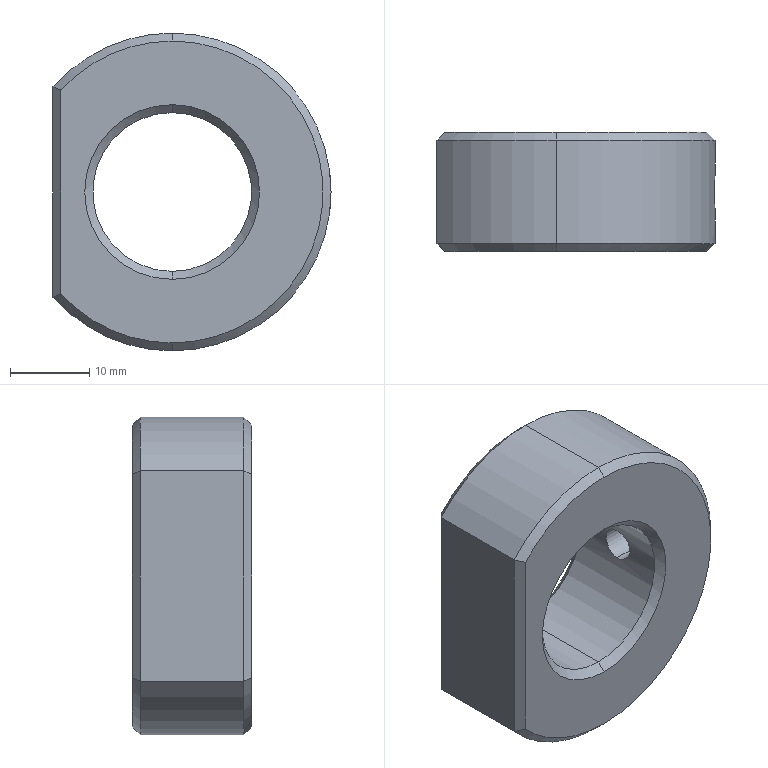Part | SolidWorks | features Chamfer 1, Extrusion 1, HoleWzd 1, ICE 1 | 1 solid | 22 faces | box 35 x 15 x 40 mm | volume 12452 mm3 | cone 10 | cylinder 7 | plane 5 | commonest cylinder face diameters 40 x3 4.2 x2 20 x2
STEP:
#1=CARTESIAN_POINT('',(19.889,7.5,-2.1));
#2=VERTEX_POINT('',#1);
#3=CARTESIAN_POINT('',(19.889,7.5,2.1));
#4=VERTEX_POINT('',#3);
#5=CARTESIAN_POINT('',(19.889,7.5,-2.1));
#6=CARTESIAN_POINT('',(19.889,7.361,-2.1));
#7=CARTESIAN_POINT('',(19.891,7.225,-2.086));
#8=CARTESIAN_POINT('',(19.896,6.956,-2.033));
#9=CARTESIAN_POINT('',(19.901,6.823,-1.993));
#10=CARTESIAN_POINT('',(19.911,6.568,-1.887));
#11=CARTESIAN_POINT('',(19.917,6.448,-1.823));
#12=CARTESIAN_POINT('',(19.93,6.22,-1.67));
#13=CARTESIAN_POINT('',(19.938,6.112,-1.582));
#14=CARTESIAN_POINT('',(19.959,5.821,-1.291));
#15=CARTESIAN_POINT('',(19.974,5.665,-1.057));
#16=CARTESIAN_POINT('',(19.994,5.455,-0.552));
#17=CARTESIAN_POINT('',(20.,5.4,-0.276));
#18=CARTESIAN_POINT('',(20.,5.4,0.1404));
#19=CARTESIAN_POINT('',(19.999,5.414,0.2768));
#20=CARTESIAN_POINT('',(19.993,5.467,0.5453));
#21=CARTESIAN_POINT('',(19.989,5.508,0.6787));
#22=CARTESIAN_POINT('',(19.979,5.614,0.9328));
#23=CARTESIAN_POINT('',(19.973,5.678,1.053));
#24=CARTESIAN_POINT('',(19.959,5.831,1.281));
#25=CARTESIAN_POINT('',(19.952,5.919,1.389));
#26=CARTESIAN_POINT('',(19.93,6.21,1.679));
#27=CARTESIAN_POINT('',(19.916,6.444,1.836));
#28=CARTESIAN_POINT('',(19.895,6.949,2.045));
#29=CARTESIAN_POINT('',(19.889,7.226,2.1));
#30=CARTESIAN_POINT('',(19.889,7.5,2.1));
#31=B_SPLINE_CURVE_WITH_KNOTS('',3,(#5,#6,#7,#8,#9,#10,#11,#12,#13,#14,#15,#16,#17,#18,#19,#20,#21,#22,#23,#24,#25,#26,#27,#28,#29,#30),.UNSPECIFIED.,.F.,.F.,(4,2,2,2,2,2,2,2,2,2,2,2,4),(0.009856,0.01027,0.01068,0.01109,0.0115,0.01232,0.01314,0.01355,0.01396,0.01437,0.01478,0.0156,0.01642),.UNSPECIFIED.);
#32=EDGE_CURVE('',#2,#4,#31,.T.);
#33=ORIENTED_EDGE('',*,*,#32,.F.);
#34=CARTESIAN_POINT('',(9.777,7.5,-2.1));
#35=VERTEX_POINT('',#34);
#36=CARTESIAN_POINT('',(0.,7.5,-2.1));
#37=DIRECTION('',(-1.,0.,0.));
#38=VECTOR('',#37,1000.);
#39=LINE('',#36,#38);
#40=EDGE_CURVE('',#2,#35,#39,.T.);
#41=ORIENTED_EDGE('',*,*,#40,.T.);
#42=CARTESIAN_POINT('',(9.777,7.5,2.1));
#43=VERTEX_POINT('',#42);
#44=CARTESIAN_POINT('',(9.777,7.5,-2.1));
#45=CARTESIAN_POINT('',(9.777,7.226,-2.1));
#46=CARTESIAN_POINT('',(9.789,6.949,-2.045));
#47=CARTESIAN_POINT('',(9.82,6.569,-1.887));
#48=CARTESIAN_POINT('',(9.833,6.447,-1.822));
#49=CARTESIAN_POINT('',(9.86,6.218,-1.669));
#50=CARTESIAN_POINT('',(9.874,6.113,-1.583));
#51=CARTESIAN_POINT('',(9.904,5.919,-1.389));
#52=CARTESIAN_POINT('',(9.918,5.831,-1.281));
#53=CARTESIAN_POINT('',(9.945,5.679,-1.054));
#54=CARTESIAN_POINT('',(9.957,5.614,-0.9337));
#55=CARTESIAN_POINT('',(9.988,5.455,-0.5514));
#56=CARTESIAN_POINT('',(10.,5.4,-0.2782));
#57=CARTESIAN_POINT('',(10.,5.4,0.1376));
#58=CARTESIAN_POINT('',(9.997,5.413,0.2742));
#59=CARTESIAN_POINT('',(9.986,5.467,0.5435));
#60=CARTESIAN_POINT('',(9.978,5.508,0.6774));
#61=CARTESIAN_POINT('',(9.957,5.613,0.931));
#62=CARTESIAN_POINT('',(9.945,5.677,1.052));
#63=CARTESIAN_POINT('',(9.918,5.83,1.28));
#64=CARTESIAN_POINT('',(9.904,5.918,1.388));
#65=CARTESIAN_POINT('',(9.86,6.207,1.677));
#66=CARTESIAN_POINT('',(9.831,6.441,1.834));
#67=CARTESIAN_POINT('',(9.8,6.819,1.991));
#68=CARTESIAN_POINT('',(9.791,6.953,2.032));
#69=CARTESIAN_POINT('',(9.78,7.224,2.086));
#70=CARTESIAN_POINT('',(9.777,7.361,2.1));
#71=CARTESIAN_POINT('',(9.777,7.5,2.1));
#72=B_SPLINE_CURVE_WITH_KNOTS('',3,(#44,#45,#46,#47,#48,#49,#50,#51,#52,#53,#54,#55,#56,#57,#58,#59,#60,#61,#62,#63,#64,#65,#66,#67,#68,#69,#70,#71),.UNSPECIFIED.,.F.,.F.,(4,2,2,2,2,2,2,2,2,2,2,2,2,4),(0.006584,0.007407,0.007818,0.008229,0.008641,0.009052,0.009875,0.01029,0.0107,0.01111,0.01152,0.01234,0.01275,0.01317),.UNSPECIFIED.);
#73=EDGE_CURVE('',#35,#43,#72,.T.);
#74=ORIENTED_EDGE('',*,*,#73,.T.);
#75=CARTESIAN_POINT('',(0.,7.5,2.1));
#76=DIRECTION('',(-1.,0.,0.));
#77=VECTOR('',#76,1000.);
#78=LINE('',#75,#77);
#79=EDGE_CURVE('',#4,#43,#78,.T.);
#80=ORIENTED_EDGE('',*,*,#79,.F.);
#81=EDGE_LOOP('',(#33,#41,#74,#80));
#82=FACE_OUTER_BOUND('',#81,.T.);
#83=CARTESIAN_POINT('',(0.,7.5,0.));
#84=DIRECTION('',(-1.,0.,0.));
#85=DIRECTION('',(0.,0.,1.));
#86=AXIS2_PLACEMENT_3D('',#83,#84,#85);
#87=CYLINDRICAL_SURFACE('',#86,2.1);
#88=ADVANCED_FACE('',(#82),#87,.F.);
#89=CARTESIAN_POINT('',(0.,15.,19.));
#90=VERTEX_POINT('',#89);
#91=CARTESIAN_POINT('',(0.,15.,-19.));
#92=VERTEX_POINT('',#91);
#93=CARTESIAN_POINT('',(0.,15.,0.));
#94=DIRECTION('',(0.,1.,0.));
#95=DIRECTION('',(0.,0.,1.));
#96=AXIS2_PLACEMENT_3D('',#93,#94,#95);
#97=CIRCLE('',#96,19.);
#98=EDGE_CURVE('',#90,#92,#97,.T.);
#99=ORIENTED_EDGE('',*,*,#98,.F.);
#100=CARTESIAN_POINT('',(0.,14.,20.));
#101=VERTEX_POINT('',#100);
#102=CARTESIAN_POINT('',(0.,15.,19.));
#103=DIRECTION('',(0.,-0.7071,0.7071));
#104=VECTOR('',#103,1000.);
#105=LINE('',#102,#104);
#106=EDGE_CURVE('',#90,#101,#105,.T.);
#107=ORIENTED_EDGE('',*,*,#106,.T.);
#108=CARTESIAN_POINT('',(0.,14.,-20.));
#109=VERTEX_POINT('',#108);
#110=CARTESIAN_POINT('',(0.,14.,0.));
#111=DIRECTION('',(0.,-1.,0.));
#112=DIRECTION('',(0.,0.,1.));
#113=AXIS2_PLACEMENT_3D('',#110,#111,#112);
#114=CIRCLE('',#113,20.);
#115=EDGE_CURVE('',#109,#101,#114,.T.);
#116=ORIENTED_EDGE('',*,*,#115,.F.);
#117=CARTESIAN_POINT('',(0.,15.,-19.));
#118=DIRECTION('',(0.,-0.7071,-0.7071));
#119=VECTOR('',#118,1000.);
#120=LINE('',#117,#119);
#121=EDGE_CURVE('',#92,#109,#120,.T.);
#122=ORIENTED_EDGE('',*,*,#121,.F.);
#123=EDGE_LOOP('',(#99,#107,#116,#122));
#124=FACE_OUTER_BOUND('',#123,.T.);
#125=CARTESIAN_POINT('',(0.,15.,0.));
#126=DIRECTION('',(0.,-1.,0.));
#127=DIRECTION('',(0.,0.,-1.));
#128=AXIS2_PLACEMENT_3D('',#125,#126,#127);
#129=CONICAL_SURFACE('',#128,19.,0.7854);
#130=ADVANCED_FACE('',(#124),#129,.T.);
#131=CARTESIAN_POINT('',(-14.,15.,-12.845));
#132=VERTEX_POINT('',#131);
#133=CARTESIAN_POINT('',(0.,15.,0.));
#134=DIRECTION('',(0.,1.,0.));
#135=DIRECTION('',(0.,0.,1.));
#136=AXIS2_PLACEMENT_3D('',#133,#134,#135);
#137=CIRCLE('',#136,19.);
#138=EDGE_CURVE('',#92,#132,#137,.T.);
#139=ORIENTED_EDGE('',*,*,#138,.F.);
#140=ORIENTED_EDGE('',*,*,#121,.T.);
#141=CARTESIAN_POINT('',(-15.,14.,-13.229));
#142=VERTEX_POINT('',#141);
#143=CARTESIAN_POINT('',(0.,14.,0.));
#144=DIRECTION('',(0.,-1.,0.));
#145=DIRECTION('',(0.,0.,1.));
#146=AXIS2_PLACEMENT_3D('',#143,#144,#145);
#147=CIRCLE('',#146,20.);
#148=EDGE_CURVE('',#142,#109,#147,.T.);
#149=ORIENTED_EDGE('',*,*,#148,.F.);
#150=CARTESIAN_POINT('',(-14.,15.,-12.845));
#151=CARTESIAN_POINT('',(-14.333,14.667,-12.975));
#152=CARTESIAN_POINT('',(-14.666,14.334,-13.103));
#153=CARTESIAN_POINT('',(-15.,14.,-13.229));
#154=B_SPLINE_CURVE_WITH_KNOTS('',3,(#150,#151,#152,#153),.UNSPECIFIED.,.F.,.F.,(4,4),(0.,0.001465),.UNSPECIFIED.);
#155=EDGE_CURVE('',#132,#142,#154,.T.);
#156=ORIENTED_EDGE('',*,*,#155,.F.);
#157=EDGE_LOOP('',(#139,#140,#149,#156));
#158=FACE_OUTER_BOUND('',#157,.T.);
#159=CARTESIAN_POINT('',(0.,15.,0.));
#160=DIRECTION('',(0.,-1.,0.));
#161=DIRECTION('',(0.,0.,-1.));
#162=AXIS2_PLACEMENT_3D('',#159,#160,#161);
#163=CONICAL_SURFACE('',#162,19.,0.7854);
#164=ADVANCED_FACE('',(#158),#163,.T.);
#165=CARTESIAN_POINT('',(0.,0.,-19.));
#166=VERTEX_POINT('',#165);
#167=CARTESIAN_POINT('',(0.,0.,19.));
#168=VERTEX_POINT('',#167);
#169=CARTESIAN_POINT('',(0.,0.,0.));
#170=DIRECTION('',(0.,-1.,0.));
#171=DIRECTION('',(0.,0.,1.));
#172=AXIS2_PLACEMENT_3D('',#169,#170,#171);
#173=CIRCLE('',#172,19.);
#174=EDGE_CURVE('',#166,#168,#173,.T.);
#175=ORIENTED_EDGE('',*,*,#174,.F.);
#176=CARTESIAN_POINT('',(0.,1.,-20.));
#177=VERTEX_POINT('',#176);
#178=CARTESIAN_POINT('',(0.,1.,-20.));
#179=DIRECTION('',(0.,0.7071,-0.7071));
#180=VECTOR('',#179,1000.);
#181=LINE('',#178,#180);
#182=EDGE_CURVE('',#166,#177,#181,.T.);
#183=ORIENTED_EDGE('',*,*,#182,.T.);
#184=CARTESIAN_POINT('',(0.,1.,20.));
#185=VERTEX_POINT('',#184);
#186=CARTESIAN_POINT('',(0.,1.,0.));
#187=DIRECTION('',(0.,1.,0.));
#188=DIRECTION('',(0.,0.,1.));
#189=AXIS2_PLACEMENT_3D('',#186,#187,#188);
#190=CIRCLE('',#189,20.);
#191=EDGE_CURVE('',#185,#177,#190,.T.);
#192=ORIENTED_EDGE('',*,*,#191,.F.);
#193=CARTESIAN_POINT('',(0.,1.,20.));
#194=DIRECTION('',(0.,0.7071,0.7071));
#195=VECTOR('',#194,1000.);
#196=LINE('',#193,#195);
#197=EDGE_CURVE('',#168,#185,#196,.T.);
#198=ORIENTED_EDGE('',*,*,#197,.F.);
#199=EDGE_LOOP('',(#175,#183,#192,#198));
#200=FACE_OUTER_BOUND('',#199,.T.);
#201=CARTESIAN_POINT('',(0.,1.,0.));
#202=DIRECTION('',(0.,1.,0.));
#203=DIRECTION('',(0.,0.,1.));
#204=AXIS2_PLACEMENT_3D('',#201,#202,#203);
#205=CONICAL_SURFACE('',#204,20.,0.7854);
#206=ADVANCED_FACE('',(#200),#205,.T.);
#207=CARTESIAN_POINT('',(-14.,0.,12.845));
#208=VERTEX_POINT('',#207);
#209=CARTESIAN_POINT('',(0.,0.,0.));
#210=DIRECTION('',(0.,-1.,0.));
#211=DIRECTION('',(0.,0.,1.));
#212=AXIS2_PLACEMENT_3D('',#209,#210,#211);
#213=CIRCLE('',#212,19.);
#214=EDGE_CURVE('',#168,#208,#213,.T.);
#215=ORIENTED_EDGE('',*,*,#214,.F.);
#216=ORIENTED_EDGE('',*,*,#197,.T.);
#217=CARTESIAN_POINT('',(-15.,1.,13.229));
#218=VERTEX_POINT('',#217);
#219=CARTESIAN_POINT('',(0.,1.,0.));
#220=DIRECTION('',(0.,1.,0.));
#221=DIRECTION('',(0.,0.,1.));
#222=AXIS2_PLACEMENT_3D('',#219,#220,#221);
#223=CIRCLE('',#222,20.);
#224=EDGE_CURVE('',#218,#185,#223,.T.);
#225=ORIENTED_EDGE('',*,*,#224,.F.);
#226=CARTESIAN_POINT('',(-14.,0.,12.845));
#227=CARTESIAN_POINT('',(-14.333,0.333,12.975));
#228=CARTESIAN_POINT('',(-14.666,0.6663,13.103));
#229=CARTESIAN_POINT('',(-15.,1.,13.229));
#230=B_SPLINE_CURVE_WITH_KNOTS('',3,(#226,#227,#228,#229),.UNSPECIFIED.,.F.,.F.,(4,4),(0.,0.001465),.UNSPECIFIED.);
#231=EDGE_CURVE('',#208,#218,#230,.T.);
#232=ORIENTED_EDGE('',*,*,#231,.F.);
#233=EDGE_LOOP('',(#215,#216,#225,#232));
#234=FACE_OUTER_BOUND('',#233,.T.);
#235=CARTESIAN_POINT('',(0.,1.,0.));
#236=DIRECTION('',(0.,1.,0.));
#237=DIRECTION('',(0.,0.,1.));
#238=AXIS2_PLACEMENT_3D('',#235,#236,#237);
#239=CONICAL_SURFACE('',#238,20.,0.7854);
#240=ADVANCED_FACE('',(#234),#239,.T.);
#241=CARTESIAN_POINT('',(0.,14.,-10.));
#242=VERTEX_POINT('',#241);
#243=CARTESIAN_POINT('',(0.,14.,10.));
#244=VERTEX_POINT('',#243);
#245=CARTESIAN_POINT('',(0.,14.,0.));
#246=DIRECTION('',(0.,1.,0.));
#247=DIRECTION('',(0.,0.,1.));
#248=AXIS2_PLACEMENT_3D('',#245,#246,#247);
#249=CIRCLE('',#248,10.);
#250=EDGE_CURVE('',#242,#244,#249,.T.);
#251=ORIENTED_EDGE('',*,*,#250,.F.);
#252=CARTESIAN_POINT('',(0.,15.,-11.));
#253=VERTEX_POINT('',#252);
#254=CARTESIAN_POINT('',(0.,14.,-10.));
#255=DIRECTION('',(0.,0.7071,-0.7071));
#256=VECTOR('',#255,1000.);
#257=LINE('',#254,#256);
#258=EDGE_CURVE('',#242,#253,#257,.T.);
#259=ORIENTED_EDGE('',*,*,#258,.T.);
#260=CARTESIAN_POINT('',(0.,15.,11.));
#261=VERTEX_POINT('',#260);
#262=CARTESIAN_POINT('',(0.,15.,0.));
#263=DIRECTION('',(0.,-1.,0.));
#264=DIRECTION('',(0.,0.,1.));
#265=AXIS2_PLACEMENT_3D('',#262,#263,#264);
#266=CIRCLE('',#265,11.);
#267=EDGE_CURVE('',#261,#253,#266,.T.);
#268=ORIENTED_EDGE('',*,*,#267,.F.);
#269=CARTESIAN_POINT('',(0.,14.,10.));
#270=DIRECTION('',(0.,0.7071,0.7071));
#271=VECTOR('',#270,1000.);
#272=LINE('',#269,#271);
#273=EDGE_CURVE('',#244,#261,#272,.T.);
#274=ORIENTED_EDGE('',*,*,#273,.F.);
#275=EDGE_LOOP('',(#251,#259,#268,#274));
#276=FACE_OUTER_BOUND('',#275,.T.);
#277=CARTESIAN_POINT('',(0.,14.,0.));
#278=DIRECTION('',(0.,1.,0.));
#279=DIRECTION('',(0.,0.,1.));
#280=AXIS2_PLACEMENT_3D('',#277,#278,#279);
#281=CONICAL_SURFACE('',#280,10.,0.7854);
#282=ADVANCED_FACE('',(#276),#281,.F.);
#283=CARTESIAN_POINT('',(0.,1.,10.));
#284=VERTEX_POINT('',#283);
#285=CARTESIAN_POINT('',(0.,1.,-10.));
#286=VERTEX_POINT('',#285);
#287=CARTESIAN_POINT('',(0.,1.,0.));
#288=DIRECTION('',(0.,-1.,0.));
#289=DIRECTION('',(0.,0.,1.));
#290=AXIS2_PLACEMENT_3D('',#287,#288,#289);
#291=CIRCLE('',#290,10.);
#292=EDGE_CURVE('',#284,#286,#291,.T.);
#293=ORIENTED_EDGE('',*,*,#292,.F.);
#294=CARTESIAN_POINT('',(0.,0.,11.));
#295=VERTEX_POINT('',#294);
#296=CARTESIAN_POINT('',(0.,0.,11.));
#297=DIRECTION('',(0.,-0.7071,0.7071));
#298=VECTOR('',#297,1000.);
#299=LINE('',#296,#298);
#300=EDGE_CURVE('',#284,#295,#299,.T.);
#301=ORIENTED_EDGE('',*,*,#300,.T.);
#302=CARTESIAN_POINT('',(0.,0.,-11.));
#303=VERTEX_POINT('',#302);
#304=CARTESIAN_POINT('',(0.,0.,0.));
#305=DIRECTION('',(0.,1.,0.));
#306=DIRECTION('',(0.,0.,1.));
#307=AXIS2_PLACEMENT_3D('',#304,#305,#306);
#308=CIRCLE('',#307,11.);
#309=EDGE_CURVE('',#303,#295,#308,.T.);
#310=ORIENTED_EDGE('',*,*,#309,.F.);
#311=CARTESIAN_POINT('',(0.,0.,-11.));
#312=DIRECTION('',(0.,-0.7071,-0.7071));
#313=VECTOR('',#312,1000.);
#314=LINE('',#311,#313);
#315=EDGE_CURVE('',#286,#303,#314,.T.);
#316=ORIENTED_EDGE('',*,*,#315,.F.);
#317=EDGE_LOOP('',(#293,#301,#310,#316));
#318=FACE_OUTER_BOUND('',#317,.T.);
#319=CARTESIAN_POINT('',(0.,0.,0.));
#320=DIRECTION('',(0.,-1.,0.));
#321=DIRECTION('',(0.,0.,-1.));
#322=AXIS2_PLACEMENT_3D('',#319,#320,#321);
#323=CONICAL_SURFACE('',#322,11.,0.7854);
#324=ADVANCED_FACE('',(#318),#323,.F.);
#325=ORIENTED_EDGE('',*,*,#250,.T.);
#326=CARTESIAN_POINT('',(0.,15.,10.));
#327=DIRECTION('',(0.,-1.,0.));
#328=VECTOR('',#327,1000.);
#329=LINE('',#326,#328);
#330=EDGE_CURVE('',#244,#284,#329,.T.);
#331=ORIENTED_EDGE('',*,*,#330,.T.);
#332=ORIENTED_EDGE('',*,*,#292,.T.);
#333=CARTESIAN_POINT('',(0.,15.,-10.));
#334=DIRECTION('',(0.,-1.,0.));
#335=VECTOR('',#334,1000.);
#336=LINE('',#333,#335);
#337=EDGE_CURVE('',#242,#286,#336,.T.);
#338=ORIENTED_EDGE('',*,*,#337,.F.);
#339=EDGE_LOOP('',(#325,#331,#332,#338));
#340=FACE_OUTER_BOUND('',#339,.T.);
#341=CARTESIAN_POINT('',(0.,15.,0.));
#342=DIRECTION('',(0.,-1.,0.));
#343=DIRECTION('',(0.,0.,-1.));
#344=AXIS2_PLACEMENT_3D('',#341,#342,#343);
#345=CYLINDRICAL_SURFACE('',#344,10.);
#346=ADVANCED_FACE('',(#340),#345,.F.);
#347=CARTESIAN_POINT('',(19.889,7.5,2.1));
#348=CARTESIAN_POINT('',(19.889,7.637,2.1));
#349=CARTESIAN_POINT('',(19.891,7.776,2.086));
#350=CARTESIAN_POINT('',(19.896,8.046,2.033));
#351=CARTESIAN_POINT('',(19.901,8.177,1.993));
#352=CARTESIAN_POINT('',(19.911,8.431,1.887));
#353=CARTESIAN_POINT('',(19.917,8.554,1.822));
#354=CARTESIAN_POINT('',(19.93,8.781,1.669));
#355=CARTESIAN_POINT('',(19.938,8.887,1.583));
#356=CARTESIAN_POINT('',(19.952,9.083,1.387));
#357=CARTESIAN_POINT('',(19.959,9.17,1.281));
#358=CARTESIAN_POINT('',(19.973,9.322,1.053));
#359=CARTESIAN_POINT('',(19.979,9.388,0.9302));
#360=CARTESIAN_POINT('',(19.989,9.493,0.6759));
#361=CARTESIAN_POINT('',(19.993,9.533,0.5449));
#362=CARTESIAN_POINT('',(19.999,9.586,0.2756));
#363=CARTESIAN_POINT('',(20.,9.6,0.1363));
#364=CARTESIAN_POINT('',(20.,9.6,-0.275));
#365=CARTESIAN_POINT('',(19.994,9.545,-0.5515));
#366=CARTESIAN_POINT('',(19.974,9.335,-1.057));
#367=CARTESIAN_POINT('',(19.959,9.179,-1.291));
#368=CARTESIAN_POINT('',(19.938,8.888,-1.582));
#369=CARTESIAN_POINT('',(19.93,8.78,-1.67));
#370=CARTESIAN_POINT('',(19.917,8.552,-1.823));
#371=CARTESIAN_POINT('',(19.911,8.432,-1.887));
#372=CARTESIAN_POINT('',(19.901,8.177,-1.993));
#373=CARTESIAN_POINT('',(19.896,8.044,-2.033));
#374=CARTESIAN_POINT('',(19.891,7.775,-2.086));
#375=CARTESIAN_POINT('',(19.889,7.639,-2.1));
#376=CARTESIAN_POINT('',(19.889,7.5,-2.1));
#377=B_SPLINE_CURVE_WITH_KNOTS('',3,(#347,#348,#349,#350,#351,#352,#353,#354,#355,#356,#357,#358,#359,#360,#361,#362,#363,#364,#365,#366,#367,#368,#369,#370,#371,#372,#373,#374,#375,#376),.UNSPECIFIED.,.F.,.F.,(4,2,2,2,2,2,2,2,2,2,2,2,2,2,4),(0.003286,0.003696,0.004107,0.004518,0.004928,0.005339,0.00575,0.00616,0.006571,0.007392,0.008213,0.008624,0.009035,0.009445,0.009856),.UNSPECIFIED.);
#378=EDGE_CURVE('',#4,#2,#377,.T.);
#379=ORIENTED_EDGE('',*,*,#378,.T.);
#380=ORIENTED_EDGE('',*,*,#32,.T.);
#381=EDGE_LOOP('',(#379,#380));
#382=FACE_BOUND('',#381,.T.);
#383=ORIENTED_EDGE('',*,*,#115,.T.);
#384=CARTESIAN_POINT('',(0.,15.,20.));
#385=DIRECTION('',(0.,-1.,0.));
#386=VECTOR('',#385,1000.);
#387=LINE('',#384,#386);
#388=EDGE_CURVE('',#101,#185,#387,.T.);
#389=ORIENTED_EDGE('',*,*,#388,.T.);
#390=ORIENTED_EDGE('',*,*,#191,.T.);
#391=CARTESIAN_POINT('',(0.,15.,-20.));
#392=DIRECTION('',(0.,-1.,0.));
#393=VECTOR('',#392,1000.);
#394=LINE('',#391,#393);
#395=EDGE_CURVE('',#109,#177,#394,.T.);
#396=ORIENTED_EDGE('',*,*,#395,.F.);
#397=EDGE_LOOP('',(#383,#389,#390,#396));
#398=FACE_OUTER_BOUND('',#397,.T.);
#399=CARTESIAN_POINT('',(0.,15.,0.));
#400=DIRECTION('',(0.,-1.,0.));
#401=DIRECTION('',(0.,0.,-1.));
#402=AXIS2_PLACEMENT_3D('',#399,#400,#401);
#403=CYLINDRICAL_SURFACE('',#402,20.);
#404=ADVANCED_FACE('',(#382,#398),#403,.T.);
#405=ORIENTED_EDGE('',*,*,#148,.T.);
#406=ORIENTED_EDGE('',*,*,#395,.T.);
#407=CARTESIAN_POINT('',(-15.,1.,-13.229));
#408=VERTEX_POINT('',#407);
#409=CARTESIAN_POINT('',(0.,1.,0.));
#410=DIRECTION('',(0.,1.,0.));
#411=DIRECTION('',(0.,0.,1.));
#412=AXIS2_PLACEMENT_3D('',#409,#410,#411);
#413=CIRCLE('',#412,20.);
#414=EDGE_CURVE('',#177,#408,#413,.T.);
#415=ORIENTED_EDGE('',*,*,#414,.T.);
#416=CARTESIAN_POINT('',(-15.,15.,-13.229));
#417=DIRECTION('',(0.,1.,0.));
#418=VECTOR('',#417,1000.);
#419=LINE('',#416,#418);
#420=EDGE_CURVE('',#408,#142,#419,.T.);
#421=ORIENTED_EDGE('',*,*,#420,.T.);
#422=EDGE_LOOP('',(#405,#406,#415,#421));
#423=FACE_OUTER_BOUND('',#422,.T.);
#424=CARTESIAN_POINT('',(0.,15.,0.));
#425=DIRECTION('',(0.,-1.,0.));
#426=DIRECTION('',(0.,0.,-1.));
#427=AXIS2_PLACEMENT_3D('',#424,#425,#426);
#428=CYLINDRICAL_SURFACE('',#427,20.);
#429=ADVANCED_FACE('',(#423),#428,.T.);
#430=ORIENTED_EDGE('',*,*,#267,.T.);
#431=CARTESIAN_POINT('',(0.,15.,0.));
#432=DIRECTION('',(0.,-1.,0.));
#433=DIRECTION('',(0.,0.,1.));
#434=AXIS2_PLACEMENT_3D('',#431,#432,#433);
#435=CIRCLE('',#434,11.);
#436=EDGE_CURVE('',#253,#261,#435,.T.);
#437=ORIENTED_EDGE('',*,*,#436,.T.);
#438=EDGE_LOOP('',(#430,#437));
#439=FACE_BOUND('',#438,.T.);
#440=CARTESIAN_POINT('',(-14.,15.,12.845));
#441=VERTEX_POINT('',#440);
#442=CARTESIAN_POINT('',(0.,15.,0.));
#443=DIRECTION('',(0.,1.,0.));
#444=DIRECTION('',(0.,0.,1.));
#445=AXIS2_PLACEMENT_3D('',#442,#443,#444);
#446=CIRCLE('',#445,19.);
#447=EDGE_CURVE('',#441,#90,#446,.T.);
#448=ORIENTED_EDGE('',*,*,#447,.T.);
#449=ORIENTED_EDGE('',*,*,#98,.T.);
#450=ORIENTED_EDGE('',*,*,#138,.T.);
#451=CARTESIAN_POINT('',(-14.,15.,13.229));
#452=DIRECTION('',(0.,0.,1.));
#453=VECTOR('',#452,1000.);
#454=LINE('',#451,#453);
#455=EDGE_CURVE('',#132,#441,#454,.T.);
#456=ORIENTED_EDGE('',*,*,#455,.T.);
#457=EDGE_LOOP('',(#448,#449,#450,#456));
#458=FACE_OUTER_BOUND('',#457,.T.);
#459=CARTESIAN_POINT('',(0.,15.,0.));
#460=DIRECTION('',(0.,1.,0.));
#461=DIRECTION('',(0.,0.,1.));
#462=AXIS2_PLACEMENT_3D('',#459,#460,#461);
#463=PLANE('',#462);
#464=ADVANCED_FACE('',(#439,#458),#463,.T.);
#465=ORIENTED_EDGE('',*,*,#309,.T.);
#466=CARTESIAN_POINT('',(0.,0.,0.));
#467=DIRECTION('',(0.,1.,0.));
#468=DIRECTION('',(0.,0.,1.));
#469=AXIS2_PLACEMENT_3D('',#466,#467,#468);
#470=CIRCLE('',#469,11.);
#471=EDGE_CURVE('',#295,#303,#470,.T.);
#472=ORIENTED_EDGE('',*,*,#471,.T.);
#473=EDGE_LOOP('',(#465,#472));
#474=FACE_BOUND('',#473,.T.);
#475=CARTESIAN_POINT('',(-14.,0.,-12.845));
#476=VERTEX_POINT('',#475);
#477=CARTESIAN_POINT('',(0.,0.,0.));
#478=DIRECTION('',(0.,-1.,0.));
#479=DIRECTION('',(0.,0.,1.));
#480=AXIS2_PLACEMENT_3D('',#477,#478,#479);
#481=CIRCLE('',#480,19.);
#482=EDGE_CURVE('',#476,#166,#481,.T.);
#483=ORIENTED_EDGE('',*,*,#482,.T.);
#484=ORIENTED_EDGE('',*,*,#174,.T.);
#485=ORIENTED_EDGE('',*,*,#214,.T.);
#486=CARTESIAN_POINT('',(-14.,0.,0.));
#487=DIRECTION('',(0.,0.,-1.));
#488=VECTOR('',#487,1000.);
#489=LINE('',#486,#488);
#490=EDGE_CURVE('',#208,#476,#489,.T.);
#491=ORIENTED_EDGE('',*,*,#490,.T.);
#492=EDGE_LOOP('',(#483,#484,#485,#491));
#493=FACE_OUTER_BOUND('',#492,.T.);
#494=CARTESIAN_POINT('',(0.,0.,0.));
#495=DIRECTION('',(0.,1.,0.));
#496=DIRECTION('',(0.,0.,1.));
#497=AXIS2_PLACEMENT_3D('',#494,#495,#496);
#498=PLANE('',#497);
#499=ADVANCED_FACE('',(#474,#493),#498,.F.);
#500=ORIENTED_EDGE('',*,*,#388,.F.);
#501=CARTESIAN_POINT('',(-15.,14.,13.229));
#502=VERTEX_POINT('',#501);
#503=CARTESIAN_POINT('',(0.,14.,0.));
#504=DIRECTION('',(0.,-1.,0.));
#505=DIRECTION('',(0.,0.,1.));
#506=AXIS2_PLACEMENT_3D('',#503,#504,#505);
#507=CIRCLE('',#506,20.);
#508=EDGE_CURVE('',#101,#502,#507,.T.);
#509=ORIENTED_EDGE('',*,*,#508,.T.);
#510=CARTESIAN_POINT('',(-15.,15.,13.229));
#511=DIRECTION('',(0.,-1.,0.));
#512=VECTOR('',#511,1000.);
#513=LINE('',#510,#512);
#514=EDGE_CURVE('',#502,#218,#513,.T.);
#515=ORIENTED_EDGE('',*,*,#514,.T.);
#516=ORIENTED_EDGE('',*,*,#224,.T.);
#517=EDGE_LOOP('',(#500,#509,#515,#516));
#518=FACE_OUTER_BOUND('',#517,.T.);
#519=CARTESIAN_POINT('',(0.,15.,0.));
#520=DIRECTION('',(0.,-1.,0.));
#521=DIRECTION('',(0.,0.,-1.));
#522=AXIS2_PLACEMENT_3D('',#519,#520,#521);
#523=CYLINDRICAL_SURFACE('',#522,20.);
#524=ADVANCED_FACE('',(#518),#523,.T.);
#525=ORIENTED_EDGE('',*,*,#330,.F.);
#526=CARTESIAN_POINT('',(0.,14.,0.));
#527=DIRECTION('',(0.,1.,0.));
#528=DIRECTION('',(0.,0.,1.));
#529=AXIS2_PLACEMENT_3D('',#526,#527,#528);
#530=CIRCLE('',#529,10.);
#531=EDGE_CURVE('',#244,#242,#530,.T.);
#532=ORIENTED_EDGE('',*,*,#531,.T.);
#533=ORIENTED_EDGE('',*,*,#337,.T.);
#534=CARTESIAN_POINT('',(0.,1.,0.));
#535=DIRECTION('',(0.,-1.,0.));
#536=DIRECTION('',(0.,0.,1.));
#537=AXIS2_PLACEMENT_3D('',#534,#535,#536);
#538=CIRCLE('',#537,10.);
#539=EDGE_CURVE('',#286,#284,#538,.T.);
#540=ORIENTED_EDGE('',*,*,#539,.T.);
#541=EDGE_LOOP('',(#525,#532,#533,#540));
#542=FACE_OUTER_BOUND('',#541,.T.);
#543=CARTESIAN_POINT('',(9.777,7.5,2.1));
#544=CARTESIAN_POINT('',(9.777,7.639,2.1));
#545=CARTESIAN_POINT('',(9.78,7.776,2.086));
#546=CARTESIAN_POINT('',(9.791,8.045,2.033));
#547=CARTESIAN_POINT('',(9.8,8.178,1.992));
#548=CARTESIAN_POINT('',(9.821,8.433,1.887));
#549=CARTESIAN_POINT('',(9.833,8.553,1.822));
#550=CARTESIAN_POINT('',(9.86,8.781,1.67));
#551=CARTESIAN_POINT('',(9.875,8.889,1.581));
#552=CARTESIAN_POINT('',(9.918,9.178,1.291));
#553=CARTESIAN_POINT('',(9.947,9.335,1.058));
#554=CARTESIAN_POINT('',(9.978,9.492,0.6788));
#555=CARTESIAN_POINT('',(9.986,9.532,0.546));
#556=CARTESIAN_POINT('',(9.997,9.587,0.2748));
#557=CARTESIAN_POINT('',(10.,9.6,0.1382));
#558=CARTESIAN_POINT('',(10.,9.6,-0.1366));
#559=CARTESIAN_POINT('',(9.997,9.586,-0.2762));
#560=CARTESIAN_POINT('',(9.986,9.532,-0.5458));
#561=CARTESIAN_POINT('',(9.978,9.493,-0.6769));
#562=CARTESIAN_POINT('',(9.947,9.334,-1.059));
#563=CARTESIAN_POINT('',(9.918,9.18,-1.29));
#564=CARTESIAN_POINT('',(9.874,8.887,-1.583));
#565=CARTESIAN_POINT('',(9.86,8.782,-1.669));
#566=CARTESIAN_POINT('',(9.833,8.554,-1.821));
#567=CARTESIAN_POINT('',(9.82,8.431,-1.887));
#568=CARTESIAN_POINT('',(9.8,8.178,-1.992));
#569=CARTESIAN_POINT('',(9.791,8.047,-2.032));
#570=CARTESIAN_POINT('',(9.78,7.777,-2.086));
#571=CARTESIAN_POINT('',(9.777,7.637,-2.1));
#572=CARTESIAN_POINT('',(9.777,7.5,-2.1));
#573=B_SPLINE_CURVE_WITH_KNOTS('',3,(#543,#544,#545,#546,#547,#548,#549,#550,#551,#552,#553,#554,#555,#556,#557,#558,#559,#560,#561,#562,#563,#564,#565,#566,#567,#568,#569,#570,#571,#572),.UNSPECIFIED.,.F.,.F.,(4,2,2,2,2,2,2,2,2,2,2,2,2,2,4),(0.,0.0004115,0.000823,0.001234,0.001646,0.002469,0.00288,0.003292,0.003703,0.004115,0.004938,0.005349,0.005761,0.006172,0.006584),.UNSPECIFIED.);
#574=EDGE_CURVE('',#43,#35,#573,.T.);
#575=ORIENTED_EDGE('',*,*,#574,.F.);
#576=ORIENTED_EDGE('',*,*,#73,.F.);
#577=EDGE_LOOP('',(#575,#576));
#578=FACE_BOUND('',#577,.T.);
#579=CARTESIAN_POINT('',(0.,15.,0.));
#580=DIRECTION('',(0.,-1.,0.));
#581=DIRECTION('',(0.,0.,-1.));
#582=AXIS2_PLACEMENT_3D('',#579,#580,#581);
#583=CYLINDRICAL_SURFACE('',#582,10.);
#584=ADVANCED_FACE('',(#542,#578),#583,.F.);
#585=ORIENTED_EDGE('',*,*,#420,.F.);
#586=CARTESIAN_POINT('',(-15.,1.,-23.818));
#587=DIRECTION('',(0.,0.,1.));
#588=VECTOR('',#587,1000.);
#589=LINE('',#586,#588);
#590=EDGE_CURVE('',#408,#218,#589,.T.);
#591=ORIENTED_EDGE('',*,*,#590,.T.);
#592=ORIENTED_EDGE('',*,*,#514,.F.);
#593=CARTESIAN_POINT('',(-15.,14.,-13.229));
#594=DIRECTION('',(0.,0.,-1.));
#595=VECTOR('',#594,1000.);
#596=LINE('',#593,#595);
#597=EDGE_CURVE('',#502,#142,#596,.T.);
#598=ORIENTED_EDGE('',*,*,#597,.T.);
#599=EDGE_LOOP('',(#585,#591,#592,#598));
#600=FACE_OUTER_BOUND('',#599,.T.);
#601=CARTESIAN_POINT('',(-15.,0.,-23.818));
#602=DIRECTION('',(1.,0.,0.));
#603=DIRECTION('',(0.,0.,-1.));
#604=AXIS2_PLACEMENT_3D('',#601,#602,#603);
#605=PLANE('',#604);
#606=ADVANCED_FACE('',(#600),#605,.F.);
#607=ORIENTED_EDGE('',*,*,#300,.F.);
#608=ORIENTED_EDGE('',*,*,#539,.F.);
#609=ORIENTED_EDGE('',*,*,#315,.T.);
#610=ORIENTED_EDGE('',*,*,#471,.F.);
#611=EDGE_LOOP('',(#607,#608,#609,#610));
#612=FACE_OUTER_BOUND('',#611,.T.);
#613=CARTESIAN_POINT('',(0.,0.,0.));
#614=DIRECTION('',(0.,-1.,0.));
#615=DIRECTION('',(0.,0.,-1.));
#616=AXIS2_PLACEMENT_3D('',#613,#614,#615);
#617=CONICAL_SURFACE('',#616,11.,0.7854);
#618=ADVANCED_FACE('',(#612),#617,.F.);
#619=ORIENTED_EDGE('',*,*,#258,.F.);
#620=ORIENTED_EDGE('',*,*,#531,.F.);
#621=ORIENTED_EDGE('',*,*,#273,.T.);
#622=ORIENTED_EDGE('',*,*,#436,.F.);
#623=EDGE_LOOP('',(#619,#620,#621,#622));
#624=FACE_OUTER_BOUND('',#623,.T.);
#625=CARTESIAN_POINT('',(0.,14.,0.));
#626=DIRECTION('',(0.,1.,0.));
#627=DIRECTION('',(0.,0.,1.));
#628=AXIS2_PLACEMENT_3D('',#625,#626,#627);
#629=CONICAL_SURFACE('',#628,10.,0.7854);
#630=ADVANCED_FACE('',(#624),#629,.F.);
#631=ORIENTED_EDGE('',*,*,#182,.F.);
#632=ORIENTED_EDGE('',*,*,#482,.F.);
#633=CARTESIAN_POINT('',(-15.,1.,-13.229));
#634=CARTESIAN_POINT('',(-14.666,0.6663,-13.103));
#635=CARTESIAN_POINT('',(-14.333,0.333,-12.975));
#636=CARTESIAN_POINT('',(-14.,0.,-12.845));
#637=B_SPLINE_CURVE_WITH_KNOTS('',3,(#633,#634,#635,#636),.UNSPECIFIED.,.F.,.F.,(4,4),(0.,0.001465),.UNSPECIFIED.);
#638=EDGE_CURVE('',#408,#476,#637,.T.);
#639=ORIENTED_EDGE('',*,*,#638,.F.);
#640=ORIENTED_EDGE('',*,*,#414,.F.);
#641=EDGE_LOOP('',(#631,#632,#639,#640));
#642=FACE_OUTER_BOUND('',#641,.T.);
#643=CARTESIAN_POINT('',(0.,1.,0.));
#644=DIRECTION('',(0.,1.,0.));
#645=DIRECTION('',(0.,0.,1.));
#646=AXIS2_PLACEMENT_3D('',#643,#644,#645);
#647=CONICAL_SURFACE('',#646,20.,0.7854);
#648=ADVANCED_FACE('',(#642),#647,.T.);
#649=ORIENTED_EDGE('',*,*,#231,.T.);
#650=ORIENTED_EDGE('',*,*,#590,.F.);
#651=ORIENTED_EDGE('',*,*,#638,.T.);
#652=ORIENTED_EDGE('',*,*,#490,.F.);
#653=EDGE_LOOP('',(#649,#650,#651,#652));
#654=FACE_OUTER_BOUND('',#653,.T.);
#655=CARTESIAN_POINT('',(-14.,0.,0.));
#656=DIRECTION('',(0.7071,0.7071,0.));
#657=DIRECTION('',(0.,0.,-1.));
#658=AXIS2_PLACEMENT_3D('',#655,#656,#657);
#659=PLANE('',#658);
#660=ADVANCED_FACE('',(#654),#659,.F.);
#661=ORIENTED_EDGE('',*,*,#106,.F.);
#662=ORIENTED_EDGE('',*,*,#447,.F.);
#663=CARTESIAN_POINT('',(-15.,14.,13.229));
#664=CARTESIAN_POINT('',(-14.666,14.334,13.103));
#665=CARTESIAN_POINT('',(-14.333,14.667,12.975));
#666=CARTESIAN_POINT('',(-14.,15.,12.845));
#667=B_SPLINE_CURVE_WITH_KNOTS('',3,(#663,#664,#665,#666),.UNSPECIFIED.,.F.,.F.,(4,4),(0.,0.001465),.UNSPECIFIED.);
#668=EDGE_CURVE('',#502,#441,#667,.T.);
#669=ORIENTED_EDGE('',*,*,#668,.F.);
#670=ORIENTED_EDGE('',*,*,#508,.F.);
#671=EDGE_LOOP('',(#661,#662,#669,#670));
#672=FACE_OUTER_BOUND('',#671,.T.);
#673=CARTESIAN_POINT('',(0.,15.,0.));
#674=DIRECTION('',(0.,-1.,0.));
#675=DIRECTION('',(0.,0.,-1.));
#676=AXIS2_PLACEMENT_3D('',#673,#674,#675);
#677=CONICAL_SURFACE('',#676,19.,0.7854);
#678=ADVANCED_FACE('',(#672),#677,.T.);
#679=ORIENTED_EDGE('',*,*,#668,.T.);
#680=ORIENTED_EDGE('',*,*,#455,.F.);
#681=ORIENTED_EDGE('',*,*,#155,.T.);
#682=ORIENTED_EDGE('',*,*,#597,.F.);
#683=EDGE_LOOP('',(#679,#680,#681,#682));
#684=FACE_OUTER_BOUND('',#683,.T.);
#685=CARTESIAN_POINT('',(-15.,14.,-23.818));
#686=DIRECTION('',(-0.7071,0.7071,0.));
#687=DIRECTION('',(0.,0.,1.));
#688=AXIS2_PLACEMENT_3D('',#685,#686,#687);
#689=PLANE('',#688);
#690=ADVANCED_FACE('',(#684),#689,.T.);
#691=ORIENTED_EDGE('',*,*,#40,.F.);
#692=ORIENTED_EDGE('',*,*,#378,.F.);
#693=ORIENTED_EDGE('',*,*,#79,.T.);
#694=ORIENTED_EDGE('',*,*,#574,.T.);
#695=EDGE_LOOP('',(#691,#692,#693,#694));
#696=FACE_OUTER_BOUND('',#695,.T.);
#697=CARTESIAN_POINT('',(0.,7.5,0.));
#698=DIRECTION('',(-1.,0.,0.));
#699=DIRECTION('',(0.,0.,1.));
#700=AXIS2_PLACEMENT_3D('',#697,#698,#699);
#701=CYLINDRICAL_SURFACE('',#700,2.1);
#702=ADVANCED_FACE('',(#696),#701,.F.);
#703=CLOSED_SHELL('',(#88,#130,#164,#206,#240,#282,#324,#346,#404,#429,#464,#499,#524,#584,#606,#618,#630,#648,#660,#678,#690,#702));
#704=MANIFOLD_SOLID_BREP('',#703);
#705=CARTESIAN_POINT('',(0.,0.,0.));
#706=DIRECTION('',(0.,0.,1.));
#707=DIRECTION('',(1.,0.,0.));
#708=AXIS2_PLACEMENT_3D('',#705,#706,#707);
#709=(LENGTH_UNIT()NAMED_UNIT(*)SI_UNIT(.MILLI.,.METRE.));
#710=UNCERTAINTY_MEASURE_WITH_UNIT(LENGTH_MEASURE(0.00001),#709,'','');
#711=(NAMED_UNIT(*)PLANE_ANGLE_UNIT()SI_UNIT($,.RADIAN.));
#712=(NAMED_UNIT(*)SI_UNIT($,.STERADIAN.)SOLID_ANGLE_UNIT());
#713=(GEOMETRIC_REPRESENTATION_CONTEXT(3)GLOBAL_UNCERTAINTY_ASSIGNED_CONTEXT((#710))GLOBAL_UNIT_ASSIGNED_CONTEXT((#709,#711,#712))REPRESENTATION_CONTEXT('',''));
#714=ADVANCED_BREP_SHAPE_REPRESENTATION('',(#704,#708),#713);